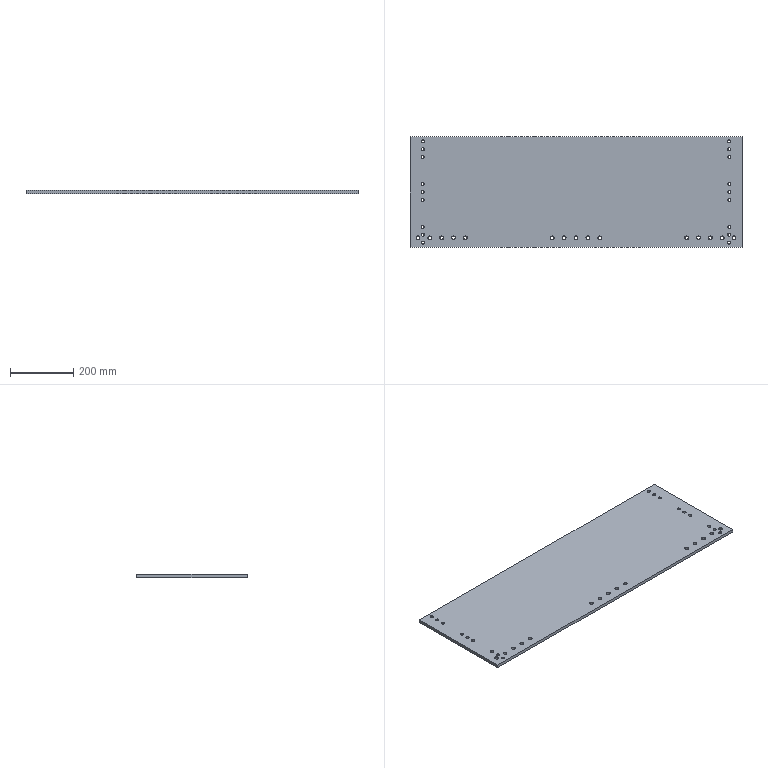Part | NX | features SIMPLE HOLE 33, SYMBOLIC_THREAD 33, DATUM_CSYS 5, SKETCH 4, HOLE PACKAGE 3, EXTRACT_FACE 2, EXTRUDE 1, Instance Feature 1, Mirror Feature 1 | 1 solid | 105 faces | box 1050 x 350 x 10 mm | volume 3649259 mm3 | cone 66 | cylinder 33 | plane 6 | commonest cylinder face diameters 9 x18 10.9 x15